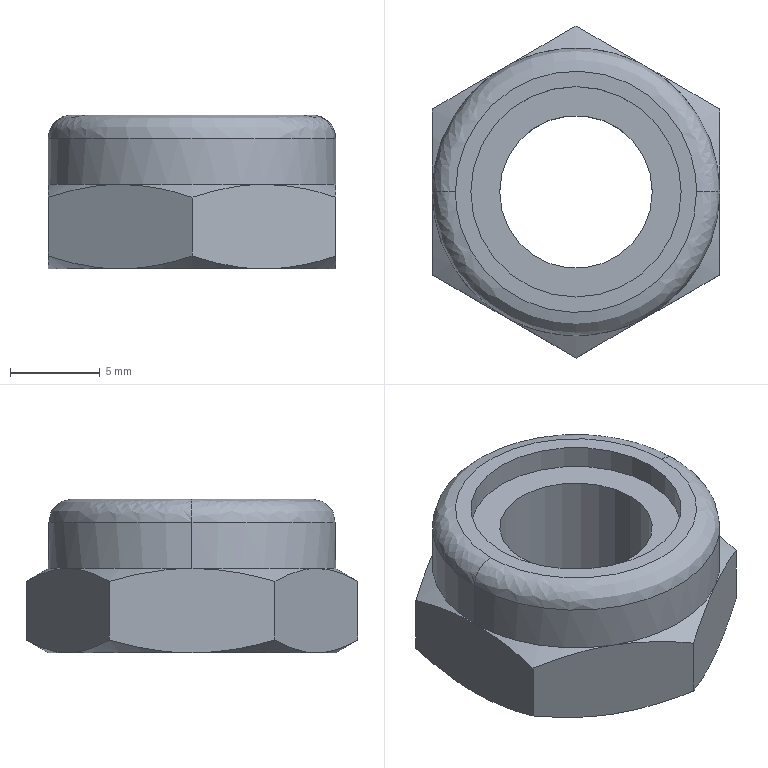Part | STEP file | Microwave Drying Flat Conveyor-prevailing torque nut thin insert_din_DIN EN ISO 10511 - M10 - N_Default | 1 solid | 33 faces | box 16 x 18.475 x 8.56 mm | volume 1235 mm3 | cone 14 | plane 9 | cylinder 8 | spline 2 | commonest cylinder face diameters 8.5 x2 10 x2 11.714 x2 16 x2
STEP:
#1=CARTESIAN_POINT('',(6.713,0.,3.86));
#2=VERTEX_POINT('',#1);
#3=CARTESIAN_POINT('',(-6.713,0.,3.86));
#4=VERTEX_POINT('',#3);
#5=CARTESIAN_POINT('',(6.713,0.,3.86));
#6=CARTESIAN_POINT('',(6.713,-13.427,3.86));
#7=CARTESIAN_POINT('',(-6.713,-13.427,3.86));
#8=CARTESIAN_POINT('',(-6.713,0.,3.86));
#9=(BOUNDED_CURVE()B_SPLINE_CURVE(3,(#5,#6,#7,#8),.UNSPECIFIED.,.F.,.F.)B_SPLINE_CURVE_WITH_KNOTS((4,4),(0.,1.),.UNSPECIFIED.)CURVE()GEOMETRIC_REPRESENTATION_ITEM()RATIONAL_B_SPLINE_CURVE((1.,0.3333,0.3333,1.))REPRESENTATION_ITEM(''));
#10=EDGE_CURVE('',#2,#4,#9,.T.);
#11=ORIENTED_EDGE('',*,*,#10,.T.);
#12=CARTESIAN_POINT('',(-8.,0.,2.573));
#13=VERTEX_POINT('',#12);
#14=CARTESIAN_POINT('',(-6.713,0.,2.573));
#15=DIRECTION('',(0.,-1.,0.));
#16=DIRECTION('',(-1.,0.,0.));
#17=AXIS2_PLACEMENT_3D('',#14,#15,#16);
#18=CIRCLE('',#17,1.287);
#19=EDGE_CURVE('',#4,#13,#18,.T.);
#20=ORIENTED_EDGE('',*,*,#19,.T.);
#21=CARTESIAN_POINT('',(8.,0.,2.573));
#22=VERTEX_POINT('',#21);
#23=CARTESIAN_POINT('',(0.,0.,2.573));
#24=DIRECTION('',(0.,0.,-1.));
#25=DIRECTION('',(1.,0.,0.));
#26=AXIS2_PLACEMENT_3D('',#23,#24,#25);
#27=CIRCLE('',#26,8.);
#28=EDGE_CURVE('',#22,#13,#27,.T.);
#29=ORIENTED_EDGE('',*,*,#28,.F.);
#30=CARTESIAN_POINT('',(6.713,0.,2.573));
#31=DIRECTION('',(0.,1.,0.));
#32=DIRECTION('',(1.,0.,0.));
#33=AXIS2_PLACEMENT_3D('',#30,#31,#32);
#34=CIRCLE('',#33,1.287);
#35=EDGE_CURVE('',#2,#22,#34,.T.);
#36=ORIENTED_EDGE('',*,*,#35,.F.);
#37=EDGE_LOOP('',(#11,#20,#29,#36));
#38=FACE_OUTER_BOUND('',#37,.T.);
#39=CARTESIAN_POINT('',(-6.713,0.,3.86));
#40=CARTESIAN_POINT('',(-6.713,-13.427,3.86));
#41=CARTESIAN_POINT('',(6.713,-13.427,3.86));
#42=CARTESIAN_POINT('',(6.713,0.,3.86));
#43=CARTESIAN_POINT('',(-7.467,0.,3.86));
#44=CARTESIAN_POINT('',(-7.467,-14.934,3.86));
#45=CARTESIAN_POINT('',(7.467,-14.934,3.86));
#46=CARTESIAN_POINT('',(7.467,0.,3.86));
#47=CARTESIAN_POINT('',(-8.,0.,3.327));
#48=CARTESIAN_POINT('',(-8.,-16.,3.327));
#49=CARTESIAN_POINT('',(8.,-16.,3.327));
#50=CARTESIAN_POINT('',(8.,0.,3.327));
#51=CARTESIAN_POINT('',(-8.,0.,2.573));
#52=CARTESIAN_POINT('',(-8.,-16.,2.573));
#53=CARTESIAN_POINT('',(8.,-16.,2.573));
#54=CARTESIAN_POINT('',(8.,0.,2.573));
#55=(BOUNDED_SURFACE()B_SPLINE_SURFACE(3,3,((#39,#40,#41,#42),(#43,#44,#45,#46),(#47,#48,#49,#50),(#51,#52,#53,#54)),.UNSPECIFIED.,.F.,.F.,.F.)B_SPLINE_SURFACE_WITH_KNOTS((4,4),(4,4),(0.,1.),(0.,1.),.UNSPECIFIED.)GEOMETRIC_REPRESENTATION_ITEM()RATIONAL_B_SPLINE_SURFACE(((1.,0.3333,0.3333,1.),(0.8047,0.2682,0.2682,0.8047),(0.8047,0.2682,0.2682,0.8047),(1.,0.3333,0.3333,1.)))REPRESENTATION_ITEM('')SURFACE());
#56=ADVANCED_FACE('',(#38),#55,.T.);
#57=CARTESIAN_POINT('',(-5.,0.,-4.7));
#58=VERTEX_POINT('',#57);
#59=CARTESIAN_POINT('',(5.,0.,-4.7));
#60=VERTEX_POINT('',#59);
#61=CARTESIAN_POINT('',(0.,0.,-4.7));
#62=DIRECTION('',(0.,0.,1.));
#63=DIRECTION('',(1.,0.,0.));
#64=AXIS2_PLACEMENT_3D('',#61,#62,#63);
#65=CIRCLE('',#64,5.);
#66=EDGE_CURVE('',#58,#60,#65,.T.);
#67=ORIENTED_EDGE('',*,*,#66,.F.);
#68=CARTESIAN_POINT('',(-5.,0.,-4.675));
#69=VERTEX_POINT('',#68);
#70=CARTESIAN_POINT('',(-5.,0.,19.05));
#71=DIRECTION('',(0.,0.,1.));
#72=VECTOR('',#71,1000.);
#73=LINE('',#70,#72);
#74=EDGE_CURVE('',#58,#69,#73,.T.);
#75=ORIENTED_EDGE('',*,*,#74,.T.);
#76=CARTESIAN_POINT('',(5.,0.,-4.675));
#77=VERTEX_POINT('',#76);
#78=CARTESIAN_POINT('',(0.,0.,-4.675));
#79=DIRECTION('',(0.,0.,-1.));
#80=DIRECTION('',(1.,0.,0.));
#81=AXIS2_PLACEMENT_3D('',#78,#79,#80);
#82=CIRCLE('',#81,5.);
#83=EDGE_CURVE('',#77,#69,#82,.T.);
#84=ORIENTED_EDGE('',*,*,#83,.F.);
#85=CARTESIAN_POINT('',(5.,0.,19.05));
#86=DIRECTION('',(0.,0.,1.));
#87=VECTOR('',#86,1000.);
#88=LINE('',#85,#87);
#89=EDGE_CURVE('',#60,#77,#88,.T.);
#90=ORIENTED_EDGE('',*,*,#89,.F.);
#91=EDGE_LOOP('',(#67,#75,#84,#90));
#92=FACE_OUTER_BOUND('',#91,.T.);
#93=CARTESIAN_POINT('',(0.,0.,19.05));
#94=DIRECTION('',(0.,0.,1.));
#95=DIRECTION('',(1.,0.,0.));
#96=AXIS2_PLACEMENT_3D('',#93,#94,#95);
#97=CYLINDRICAL_SURFACE('',#96,5.);
#98=ADVANCED_FACE('',(#92),#97,.F.);
#99=CARTESIAN_POINT('',(4.25,0.,-4.149));
#100=VERTEX_POINT('',#99);
#101=CARTESIAN_POINT('',(-4.25,0.,-4.149));
#102=VERTEX_POINT('',#101);
#103=CARTESIAN_POINT('',(0.,0.,-4.149));
#104=DIRECTION('',(0.,0.,-1.));
#105=DIRECTION('',(-1.,0.,0.));
#106=AXIS2_PLACEMENT_3D('',#103,#104,#105);
#107=CIRCLE('',#106,4.25);
#108=EDGE_CURVE('',#100,#102,#107,.T.);
#109=ORIENTED_EDGE('',*,*,#108,.F.);
#110=CARTESIAN_POINT('',(5.,0.,-4.675));
#111=DIRECTION('',(0.8192,0.,-0.5736));
#112=VECTOR('',#111,1000.);
#113=LINE('',#110,#112);
#114=EDGE_CURVE('',#100,#77,#113,.T.);
#115=ORIENTED_EDGE('',*,*,#114,.T.);
#116=ORIENTED_EDGE('',*,*,#83,.T.);
#117=CARTESIAN_POINT('',(-5.,0.,-4.675));
#118=DIRECTION('',(-0.8192,0.,-0.5736));
#119=VECTOR('',#118,1000.);
#120=LINE('',#117,#119);
#121=EDGE_CURVE('',#102,#69,#120,.T.);
#122=ORIENTED_EDGE('',*,*,#121,.F.);
#123=EDGE_LOOP('',(#109,#115,#116,#122));
#124=FACE_OUTER_BOUND('',#123,.T.);
#125=CARTESIAN_POINT('',(0.,0.,-4.675));
#126=DIRECTION('',(0.,0.,-1.));
#127=DIRECTION('',(-1.,0.,0.));
#128=AXIS2_PLACEMENT_3D('',#125,#126,#127);
#129=CONICAL_SURFACE('',#128,5.,0.9599);
#130=ADVANCED_FACE('',(#124),#129,.F.);
#131=ORIENTED_EDGE('',*,*,#108,.T.);
#132=CARTESIAN_POINT('',(-4.25,0.,2.573));
#133=VERTEX_POINT('',#132);
#134=CARTESIAN_POINT('',(-4.25,0.,-4.7));
#135=DIRECTION('',(0.,0.,1.));
#136=VECTOR('',#135,1000.);
#137=LINE('',#134,#136);
#138=EDGE_CURVE('',#102,#133,#137,.T.);
#139=ORIENTED_EDGE('',*,*,#138,.T.);
#140=CARTESIAN_POINT('',(4.25,0.,2.573));
#141=VERTEX_POINT('',#140);
#142=CARTESIAN_POINT('',(0.,0.,2.573));
#143=DIRECTION('',(0.,0.,-1.));
#144=DIRECTION('',(1.,0.,0.));
#145=AXIS2_PLACEMENT_3D('',#142,#143,#144);
#146=CIRCLE('',#145,4.25);
#147=EDGE_CURVE('',#141,#133,#146,.T.);
#148=ORIENTED_EDGE('',*,*,#147,.F.);
#149=CARTESIAN_POINT('',(4.25,0.,-4.7));
#150=DIRECTION('',(0.,0.,1.));
#151=VECTOR('',#150,1000.);
#152=LINE('',#149,#151);
#153=EDGE_CURVE('',#100,#141,#152,.T.);
#154=ORIENTED_EDGE('',*,*,#153,.F.);
#155=EDGE_LOOP('',(#131,#139,#148,#154));
#156=FACE_OUTER_BOUND('',#155,.T.);
#157=CARTESIAN_POINT('',(0.,0.,-4.7));
#158=DIRECTION('',(0.,0.,1.));
#159=DIRECTION('',(1.,0.,0.));
#160=AXIS2_PLACEMENT_3D('',#157,#158,#159);
#161=CYLINDRICAL_SURFACE('',#160,4.25);
#162=ADVANCED_FACE('',(#156),#161,.F.);
#163=CARTESIAN_POINT('',(-8.,0.,0.));
#164=VERTEX_POINT('',#163);
#165=CARTESIAN_POINT('',(-4.,6.928,0.));
#166=VERTEX_POINT('',#165);
#167=CARTESIAN_POINT('',(0.,0.,0.));
#168=DIRECTION('',(0.,0.,-1.));
#169=DIRECTION('',(-1.,0.,0.));
#170=AXIS2_PLACEMENT_3D('',#167,#168,#169);
#171=CIRCLE('',#170,8.);
#172=EDGE_CURVE('',#164,#166,#171,.T.);
#173=ORIENTED_EDGE('',*,*,#172,.F.);
#174=CARTESIAN_POINT('',(-8.,0.,9.481));
#175=DIRECTION('',(0.,0.,1.));
#176=VECTOR('',#175,1000.);
#177=LINE('',#174,#176);
#178=EDGE_CURVE('',#164,#13,#177,.T.);
#179=ORIENTED_EDGE('',*,*,#178,.T.);
#180=CARTESIAN_POINT('',(0.,0.,2.573));
#181=DIRECTION('',(0.,0.,-1.));
#182=DIRECTION('',(1.,0.,0.));
#183=AXIS2_PLACEMENT_3D('',#180,#181,#182);
#184=CIRCLE('',#183,8.);
#185=EDGE_CURVE('',#13,#22,#184,.T.);
#186=ORIENTED_EDGE('',*,*,#185,.T.);
#187=CARTESIAN_POINT('',(8.,0.,0.));
#188=VERTEX_POINT('',#187);
#189=CARTESIAN_POINT('',(8.,0.,9.481));
#190=DIRECTION('',(0.,0.,1.));
#191=VECTOR('',#190,1000.);
#192=LINE('',#189,#191);
#193=EDGE_CURVE('',#188,#22,#192,.T.);
#194=ORIENTED_EDGE('',*,*,#193,.F.);
#195=CARTESIAN_POINT('',(4.,6.928,0.));
#196=VERTEX_POINT('',#195);
#197=CARTESIAN_POINT('',(0.,0.,0.));
#198=DIRECTION('',(0.,0.,-1.));
#199=DIRECTION('',(-1.,0.,0.));
#200=AXIS2_PLACEMENT_3D('',#197,#198,#199);
#201=CIRCLE('',#200,8.);
#202=EDGE_CURVE('',#196,#188,#201,.T.);
#203=ORIENTED_EDGE('',*,*,#202,.F.);
#204=CARTESIAN_POINT('',(0.,0.,0.));
#205=DIRECTION('',(0.,0.,-1.));
#206=DIRECTION('',(-1.,0.,0.));
#207=AXIS2_PLACEMENT_3D('',#204,#205,#206);
#208=CIRCLE('',#207,8.);
#209=EDGE_CURVE('',#166,#196,#208,.T.);
#210=ORIENTED_EDGE('',*,*,#209,.F.);
#211=EDGE_LOOP('',(#173,#179,#186,#194,#203,#210));
#212=FACE_OUTER_BOUND('',#211,.T.);
#213=CARTESIAN_POINT('',(0.,0.,9.481));
#214=DIRECTION('',(0.,0.,1.));
#215=DIRECTION('',(1.,0.,0.));
#216=AXIS2_PLACEMENT_3D('',#213,#214,#215);
#217=CYLINDRICAL_SURFACE('',#216,8.);
#218=ADVANCED_FACE('',(#212),#217,.T.);
#219=CARTESIAN_POINT('',(5.857,0.,2.573));
#220=VERTEX_POINT('',#219);
#221=CARTESIAN_POINT('',(-5.857,0.,2.573));
#222=VERTEX_POINT('',#221);
#223=CARTESIAN_POINT('',(0.,0.,2.573));
#224=DIRECTION('',(0.,0.,-1.));
#225=DIRECTION('',(1.,0.,0.));
#226=AXIS2_PLACEMENT_3D('',#223,#224,#225);
#227=CIRCLE('',#226,5.857);
#228=EDGE_CURVE('',#220,#222,#227,.T.);
#229=ORIENTED_EDGE('',*,*,#228,.T.);
#230=CARTESIAN_POINT('',(-5.857,0.,3.86));
#231=VERTEX_POINT('',#230);
#232=CARTESIAN_POINT('',(-5.857,0.,9.481));
#233=DIRECTION('',(0.,0.,1.));
#234=VECTOR('',#233,1000.);
#235=LINE('',#232,#234);
#236=EDGE_CURVE('',#222,#231,#235,.T.);
#237=ORIENTED_EDGE('',*,*,#236,.T.);
#238=CARTESIAN_POINT('',(5.857,0.,3.86));
#239=VERTEX_POINT('',#238);
#240=CARTESIAN_POINT('',(0.,0.,3.86));
#241=DIRECTION('',(0.,0.,-1.));
#242=DIRECTION('',(1.,0.,0.));
#243=AXIS2_PLACEMENT_3D('',#240,#241,#242);
#244=CIRCLE('',#243,5.857);
#245=EDGE_CURVE('',#239,#231,#244,.T.);
#246=ORIENTED_EDGE('',*,*,#245,.F.);
#247=CARTESIAN_POINT('',(5.857,0.,9.481));
#248=DIRECTION('',(0.,0.,1.));
#249=VECTOR('',#248,1000.);
#250=LINE('',#247,#249);
#251=EDGE_CURVE('',#220,#239,#250,.T.);
#252=ORIENTED_EDGE('',*,*,#251,.F.);
#253=EDGE_LOOP('',(#229,#237,#246,#252));
#254=FACE_OUTER_BOUND('',#253,.T.);
#255=CARTESIAN_POINT('',(0.,0.,9.481));
#256=DIRECTION('',(0.,0.,1.));
#257=DIRECTION('',(1.,0.,0.));
#258=AXIS2_PLACEMENT_3D('',#255,#256,#257);
#259=CYLINDRICAL_SURFACE('',#258,5.857);
#260=ADVANCED_FACE('',(#254),#259,.F.);
#261=CARTESIAN_POINT('',(8.,0.,-4.7));
#262=VERTEX_POINT('',#261);
#263=CARTESIAN_POINT('',(4.,-6.928,-4.7));
#264=VERTEX_POINT('',#263);
#265=CARTESIAN_POINT('',(0.,0.,-4.7));
#266=DIRECTION('',(0.,0.,-1.));
#267=DIRECTION('',(1.,0.,0.));
#268=AXIS2_PLACEMENT_3D('',#265,#266,#267);
#269=CIRCLE('',#268,8.);
#270=EDGE_CURVE('',#262,#264,#269,.T.);
#271=ORIENTED_EDGE('',*,*,#270,.T.);
#272=CARTESIAN_POINT('',(-4.,-6.928,-4.7));
#273=VERTEX_POINT('',#272);
#274=CARTESIAN_POINT('',(0.,0.,-4.7));
#275=DIRECTION('',(0.,0.,-1.));
#276=DIRECTION('',(1.,0.,0.));
#277=AXIS2_PLACEMENT_3D('',#274,#275,#276);
#278=CIRCLE('',#277,8.);
#279=EDGE_CURVE('',#264,#273,#278,.T.);
#280=ORIENTED_EDGE('',*,*,#279,.T.);
#281=CARTESIAN_POINT('',(-8.,0.,-4.7));
#282=VERTEX_POINT('',#281);
#283=CARTESIAN_POINT('',(0.,0.,-4.7));
#284=DIRECTION('',(0.,0.,-1.));
#285=DIRECTION('',(1.,0.,0.));
#286=AXIS2_PLACEMENT_3D('',#283,#284,#285);
#287=CIRCLE('',#286,8.);
#288=EDGE_CURVE('',#273,#282,#287,.T.);
#289=ORIENTED_EDGE('',*,*,#288,.T.);
#290=CARTESIAN_POINT('',(-4.,6.928,-4.7));
#291=VERTEX_POINT('',#290);
#292=CARTESIAN_POINT('',(0.,0.,-4.7));
#293=DIRECTION('',(0.,0.,-1.));
#294=DIRECTION('',(1.,0.,0.));
#295=AXIS2_PLACEMENT_3D('',#292,#293,#294);
#296=CIRCLE('',#295,8.);
#297=EDGE_CURVE('',#282,#291,#296,.T.);
#298=ORIENTED_EDGE('',*,*,#297,.T.);
#299=CARTESIAN_POINT('',(4.,6.928,-4.7));
#300=VERTEX_POINT('',#299);
#301=CARTESIAN_POINT('',(0.,0.,-4.7));
#302=DIRECTION('',(0.,0.,-1.));
#303=DIRECTION('',(1.,0.,0.));
#304=AXIS2_PLACEMENT_3D('',#301,#302,#303);
#305=CIRCLE('',#304,8.);
#306=EDGE_CURVE('',#291,#300,#305,.T.);
#307=ORIENTED_EDGE('',*,*,#306,.T.);
#308=CARTESIAN_POINT('',(0.,0.,-4.7));
#309=DIRECTION('',(0.,0.,-1.));
#310=DIRECTION('',(1.,0.,0.));
#311=AXIS2_PLACEMENT_3D('',#308,#309,#310);
#312=CIRCLE('',#311,8.);
#313=EDGE_CURVE('',#300,#262,#312,.T.);
#314=ORIENTED_EDGE('',*,*,#313,.T.);
#315=EDGE_LOOP('',(#271,#280,#289,#298,#307,#314));
#316=FACE_OUTER_BOUND('',#315,.T.);
#317=CARTESIAN_POINT('',(0.,0.,-4.7));
#318=DIRECTION('',(0.,0.,1.));
#319=DIRECTION('',(1.,0.,0.));
#320=AXIS2_PLACEMENT_3D('',#317,#318,#319);
#321=CIRCLE('',#320,5.);
#322=EDGE_CURVE('',#60,#58,#321,.T.);
#323=ORIENTED_EDGE('',*,*,#322,.T.);
#324=ORIENTED_EDGE('',*,*,#66,.T.);
#325=EDGE_LOOP('',(#323,#324));
#326=FACE_BOUND('',#325,.T.);
#327=CARTESIAN_POINT('',(0.,9.238,-4.7));
#328=DIRECTION('',(0.,0.,-1.));
#329=DIRECTION('',(-1.,0.,0.));
#330=AXIS2_PLACEMENT_3D('',#327,#328,#329);
#331=PLANE('',#330);
#332=ADVANCED_FACE('',(#316,#326),#331,.T.);
#333=CARTESIAN_POINT('',(0.000000014,-9.238,-3.985));
#334=VERTEX_POINT('',#333);
#335=CARTESIAN_POINT('',(0.000000014,-9.238,-3.985));
#336=CARTESIAN_POINT('',(-0.6534,-8.86,-4.203));
#337=CARTESIAN_POINT('',(-1.312,-8.48,-4.383));
#338=CARTESIAN_POINT('',(-2.644,-7.711,-4.632));
#339=CARTESIAN_POINT('',(-3.317,-7.322,-4.7));
#340=CARTESIAN_POINT('',(-4.,-6.928,-4.7));
#341=B_SPLINE_CURVE_WITH_KNOTS('',3,(#335,#336,#337,#338,#339,#340),.UNSPECIFIED.,.F.,.F.,(4,2,4),(0.,0.002337,0.004674),.UNSPECIFIED.);
#342=EDGE_CURVE('',#334,#273,#341,.T.);
#343=ORIENTED_EDGE('',*,*,#342,.T.);
#344=ORIENTED_EDGE('',*,*,#279,.F.);
#345=CARTESIAN_POINT('',(4.,-6.928,-4.7));
#346=CARTESIAN_POINT('',(3.317,-7.322,-4.7));
#347=CARTESIAN_POINT('',(2.644,-7.711,-4.632));
#348=CARTESIAN_POINT('',(1.312,-8.48,-4.383));
#349=CARTESIAN_POINT('',(0.6534,-8.86,-4.203));
#350=CARTESIAN_POINT('',(0.000000014,-9.238,-3.985));
#351=B_SPLINE_CURVE_WITH_KNOTS('',3,(#345,#346,#347,#348,#349,#350),.UNSPECIFIED.,.F.,.F.,(4,2,4),(0.,0.002337,0.004674),.UNSPECIFIED.);
#352=EDGE_CURVE('',#264,#334,#351,.T.);
#353=ORIENTED_EDGE('',*,*,#352,.T.);
#354=EDGE_LOOP('',(#343,#344,#353));
#355=FACE_OUTER_BOUND('',#354,.T.);
#356=CARTESIAN_POINT('',(0.,0.,-3.981));
#357=DIRECTION('',(0.,0.,1.));
#358=DIRECTION('',(1.,0.,0.));
#359=AXIS2_PLACEMENT_3D('',#356,#357,#358);
#360=CONICAL_SURFACE('',#359,9.245,1.047);
#361=ADVANCED_FACE('',(#355),#360,.T.);
#362=ORIENTED_EDGE('',*,*,#270,.F.);
#363=CARTESIAN_POINT('',(8.,-4.619,-3.985));
#364=VERTEX_POINT('',#363);
#365=CARTESIAN_POINT('',(8.,0.,-4.7));
#366=CARTESIAN_POINT('',(8.,-0.7882,-4.7));
#367=CARTESIAN_POINT('',(8.,-1.566,-4.632));
#368=CARTESIAN_POINT('',(8.,-3.104,-4.383));
#369=CARTESIAN_POINT('',(8.,-3.864,-4.203));
#370=CARTESIAN_POINT('',(8.,-4.619,-3.985));
#371=B_SPLINE_CURVE_WITH_KNOTS('',3,(#365,#366,#367,#368,#369,#370),.UNSPECIFIED.,.F.,.F.,(4,2,4),(0.,0.002337,0.004674),.UNSPECIFIED.);
#372=EDGE_CURVE('',#262,#364,#371,.T.);
#373=ORIENTED_EDGE('',*,*,#372,.T.);
#374=CARTESIAN_POINT('',(8.,-4.619,-3.985));
#375=CARTESIAN_POINT('',(7.347,-4.996,-4.203));
#376=CARTESIAN_POINT('',(6.688,-5.376,-4.383));
#377=CARTESIAN_POINT('',(5.356,-6.145,-4.632));
#378=CARTESIAN_POINT('',(4.683,-6.534,-4.7));
#379=CARTESIAN_POINT('',(4.,-6.928,-4.7));
#380=B_SPLINE_CURVE_WITH_KNOTS('',3,(#374,#375,#376,#377,#378,#379),.UNSPECIFIED.,.F.,.F.,(4,2,4),(0.,0.002337,0.004674),.UNSPECIFIED.);
#381=EDGE_CURVE('',#364,#264,#380,.T.);
#382=ORIENTED_EDGE('',*,*,#381,.T.);
#383=EDGE_LOOP('',(#362,#373,#382));
#384=FACE_OUTER_BOUND('',#383,.T.);
#385=CARTESIAN_POINT('',(0.,0.,-3.981));
#386=DIRECTION('',(0.,0.,1.));
#387=DIRECTION('',(1.,0.,0.));
#388=AXIS2_PLACEMENT_3D('',#385,#386,#387);
#389=CONICAL_SURFACE('',#388,9.245,1.047);
#390=ADVANCED_FACE('',(#384),#389,.T.);
#391=CARTESIAN_POINT('',(8.,4.619,-3.985));
#392=VERTEX_POINT('',#391);
#393=CARTESIAN_POINT('',(8.,4.619,-3.985));
#394=CARTESIAN_POINT('',(8.,3.864,-4.203));
#395=CARTESIAN_POINT('',(8.,3.104,-4.383));
#396=CARTESIAN_POINT('',(8.,1.566,-4.632));
#397=CARTESIAN_POINT('',(8.,0.7882,-4.7));
#398=CARTESIAN_POINT('',(8.,0.,-4.7));
#399=B_SPLINE_CURVE_WITH_KNOTS('',3,(#393,#394,#395,#396,#397,#398),.UNSPECIFIED.,.F.,.F.,(4,2,4),(0.,0.002337,0.004674),.UNSPECIFIED.);
#400=EDGE_CURVE('',#392,#262,#399,.T.);
#401=ORIENTED_EDGE('',*,*,#400,.T.);
#402=ORIENTED_EDGE('',*,*,#313,.F.);
#403=CARTESIAN_POINT('',(4.,6.928,-4.7));
#404=CARTESIAN_POINT('',(4.683,6.534,-4.7));
#405=CARTESIAN_POINT('',(5.356,6.145,-4.632));
#406=CARTESIAN_POINT('',(6.688,5.376,-4.383));
#407=CARTESIAN_POINT('',(7.347,4.996,-4.203));
#408=CARTESIAN_POINT('',(8.,4.619,-3.985));
#409=B_SPLINE_CURVE_WITH_KNOTS('',3,(#403,#404,#405,#406,#407,#408),.UNSPECIFIED.,.F.,.F.,(4,2,4),(0.,0.002337,0.004674),.UNSPECIFIED.);
#410=EDGE_CURVE('',#300,#392,#409,.T.);
#411=ORIENTED_EDGE('',*,*,#410,.T.);
#412=EDGE_LOOP('',(#401,#402,#411));
#413=FACE_OUTER_BOUND('',#412,.T.);
#414=CARTESIAN_POINT('',(0.,0.,-3.981));
#415=DIRECTION('',(0.,0.,1.));
#416=DIRECTION('',(1.,0.,0.));
#417=AXIS2_PLACEMENT_3D('',#414,#415,#416);
#418=CONICAL_SURFACE('',#417,9.245,1.047);
#419=ADVANCED_FACE('',(#413),#418,.T.);
#420=CARTESIAN_POINT('',(-0.000000014,9.238,-3.985));
#421=VERTEX_POINT('',#420);
#422=CARTESIAN_POINT('',(-0.000000014,9.238,-3.985));
#423=CARTESIAN_POINT('',(0.6534,8.86,-4.203));
#424=CARTESIAN_POINT('',(1.312,8.48,-4.383));
#425=CARTESIAN_POINT('',(2.644,7.711,-4.632));
#426=CARTESIAN_POINT('',(3.317,7.322,-4.7));
#427=CARTESIAN_POINT('',(4.,6.928,-4.7));
#428=B_SPLINE_CURVE_WITH_KNOTS('',3,(#422,#423,#424,#425,#426,#427),.UNSPECIFIED.,.F.,.F.,(4,2,4),(0.,0.002337,0.004674),.UNSPECIFIED.);
#429=EDGE_CURVE('',#421,#300,#428,.T.);
#430=ORIENTED_EDGE('',*,*,#429,.T.);
#431=ORIENTED_EDGE('',*,*,#306,.F.);
#432=CARTESIAN_POINT('',(-4.,6.928,-4.7));
#433=CARTESIAN_POINT('',(-3.317,7.322,-4.7));
#434=CARTESIAN_POINT('',(-2.644,7.711,-4.632));
#435=CARTESIAN_POINT('',(-1.312,8.48,-4.383));
#436=CARTESIAN_POINT('',(-0.6534,8.86,-4.203));
#437=CARTESIAN_POINT('',(-0.000000014,9.238,-3.985));
#438=B_SPLINE_CURVE_WITH_KNOTS('',3,(#432,#433,#434,#435,#436,#437),.UNSPECIFIED.,.F.,.F.,(4,2,4),(0.,0.002337,0.004674),.UNSPECIFIED.);
#439=EDGE_CURVE('',#291,#421,#438,.T.);
#440=ORIENTED_EDGE('',*,*,#439,.T.);
#441=EDGE_LOOP('',(#430,#431,#440));
#442=FACE_OUTER_BOUND('',#441,.T.);
#443=CARTESIAN_POINT('',(0.,0.,-3.981));
#444=DIRECTION('',(0.,0.,1.));
#445=DIRECTION('',(1.,0.,0.));
#446=AXIS2_PLACEMENT_3D('',#443,#444,#445);
#447=CONICAL_SURFACE('',#446,9.245,1.047);
#448=ADVANCED_FACE('',(#442),#447,.T.);
#449=ORIENTED_EDGE('',*,*,#297,.F.);
#450=CARTESIAN_POINT('',(-8.,4.619,-3.985));
#451=VERTEX_POINT('',#450);
#452=CARTESIAN_POINT('',(-8.,0.,-4.7));
#453=CARTESIAN_POINT('',(-8.,0.7882,-4.7));
#454=CARTESIAN_POINT('',(-8.,1.566,-4.632));
#455=CARTESIAN_POINT('',(-8.,3.104,-4.383));
#456=CARTESIAN_POINT('',(-8.,3.864,-4.203));
#457=CARTESIAN_POINT('',(-8.,4.619,-3.985));
#458=B_SPLINE_CURVE_WITH_KNOTS('',3,(#452,#453,#454,#455,#456,#457),.UNSPECIFIED.,.F.,.F.,(4,2,4),(0.,0.002337,0.004674),.UNSPECIFIED.);
#459=EDGE_CURVE('',#282,#451,#458,.T.);
#460=ORIENTED_EDGE('',*,*,#459,.T.);
#461=CARTESIAN_POINT('',(-8.,4.619,-3.985));
#462=CARTESIAN_POINT('',(-7.347,4.996,-4.203));
#463=CARTESIAN_POINT('',(-6.688,5.376,-4.383));
#464=CARTESIAN_POINT('',(-5.356,6.145,-4.632));
#465=CARTESIAN_POINT('',(-4.683,6.534,-4.7));
#466=CARTESIAN_POINT('',(-4.,6.928,-4.7));
#467=B_SPLINE_CURVE_WITH_KNOTS('',3,(#461,#462,#463,#464,#465,#466),.UNSPECIFIED.,.F.,.F.,(4,2,4),(0.,0.002337,0.004674),.UNSPECIFIED.);
#468=EDGE_CURVE('',#451,#291,#467,.T.);
#469=ORIENTED_EDGE('',*,*,#468,.T.);
#470=EDGE_LOOP('',(#449,#460,#469));
#471=FACE_OUTER_BOUND('',#470,.T.);
#472=CARTESIAN_POINT('',(0.,0.,-3.981));
#473=DIRECTION('',(0.,0.,1.));
#474=DIRECTION('',(1.,0.,0.));
#475=AXIS2_PLACEMENT_3D('',#472,#473,#474);
#476=CONICAL_SURFACE('',#475,9.245,1.047);
#477=ADVANCED_FACE('',(#471),#476,.T.);
#478=CARTESIAN_POINT('',(-8.,-4.619,-3.985));
#479=VERTEX_POINT('',#478);
#480=CARTESIAN_POINT('',(-8.,-4.619,-3.985));
#481=CARTESIAN_POINT('',(-8.,-3.864,-4.203));
#482=CARTESIAN_POINT('',(-8.,-3.104,-4.383));
#483=CARTESIAN_POINT('',(-8.,-1.566,-4.632));
#484=CARTESIAN_POINT('',(-8.,-0.7882,-4.7));
#485=CARTESIAN_POINT('',(-8.,0.,-4.7));
#486=B_SPLINE_CURVE_WITH_KNOTS('',3,(#480,#481,#482,#483,#484,#485),.UNSPECIFIED.,.F.,.F.,(4,2,4),(0.,0.002337,0.004674),.UNSPECIFIED.);
#487=EDGE_CURVE('',#479,#282,#486,.T.);
#488=ORIENTED_EDGE('',*,*,#487,.T.);
#489=ORIENTED_EDGE('',*,*,#288,.F.);
#490=CARTESIAN_POINT('',(-4.,-6.928,-4.7));
#491=CARTESIAN_POINT('',(-4.683,-6.534,-4.7));
#492=CARTESIAN_POINT('',(-5.356,-6.145,-4.632));
#493=CARTESIAN_POINT('',(-6.688,-5.376,-4.383));
#494=CARTESIAN_POINT('',(-7.347,-4.996,-4.203));
#495=CARTESIAN_POINT('',(-8.,-4.619,-3.985));
#496=B_SPLINE_CURVE_WITH_KNOTS('',3,(#490,#491,#492,#493,#494,#495),.UNSPECIFIED.,.F.,.F.,(4,2,4),(0.,0.002337,0.004674),.UNSPECIFIED.);
#497=EDGE_CURVE('',#273,#479,#496,.T.);
#498=ORIENTED_EDGE('',*,*,#497,.T.);
#499=EDGE_LOOP('',(#488,#489,#498));
#500=FACE_OUTER_BOUND('',#499,.T.);
#501=CARTESIAN_POINT('',(0.,0.,-3.981));
#502=DIRECTION('',(0.,0.,1.));
#503=DIRECTION('',(1.,0.,0.));
#504=AXIS2_PLACEMENT_3D('',#501,#502,#503);
#505=CONICAL_SURFACE('',#504,9.245,1.047);
#506=ADVANCED_FACE('',(#500),#505,.T.);
#507=ORIENTED_EDGE('',*,*,#74,.F.);
#508=ORIENTED_EDGE('',*,*,#322,.F.);
#509=ORIENTED_EDGE('',*,*,#89,.T.);
#510=CARTESIAN_POINT('',(0.,0.,-4.675));
#511=DIRECTION('',(0.,0.,-1.));
#512=DIRECTION('',(1.,0.,0.));
#513=AXIS2_PLACEMENT_3D('',#510,#511,#512);
#514=CIRCLE('',#513,5.);
#515=EDGE_CURVE('',#69,#77,#514,.T.);
#516=ORIENTED_EDGE('',*,*,#515,.F.);
#517=EDGE_LOOP('',(#507,#508,#509,#516));
#518=FACE_OUTER_BOUND('',#517,.T.);
#519=CARTESIAN_POINT('',(0.,0.,19.05));
#520=DIRECTION('',(0.,0.,1.));
#521=DIRECTION('',(1.,0.,0.));
#522=AXIS2_PLACEMENT_3D('',#519,#520,#521);
#523=CYLINDRICAL_SURFACE('',#522,5.);
#524=ADVANCED_FACE('',(#518),#523,.F.);
#525=ORIENTED_EDGE('',*,*,#497,.F.);
#526=ORIENTED_EDGE('',*,*,#342,.F.);
#527=CARTESIAN_POINT('',(0.,-9.238,-0.7145));
#528=VERTEX_POINT('',#527);
#529=CARTESIAN_POINT('',(0.,-9.238,-4.7));
#530=DIRECTION('',(0.,0.,1.));
#531=VECTOR('',#530,1000.);
#532=LINE('',#529,#531);
#533=EDGE_CURVE('',#334,#528,#532,.T.);
#534=ORIENTED_EDGE('',*,*,#533,.T.);
#535=CARTESIAN_POINT('',(-4.,-6.928,0.));
#536=VERTEX_POINT('',#535);
#537=CARTESIAN_POINT('',(0.,-9.238,-0.7145));
#538=CARTESIAN_POINT('',(-0.6534,-8.86,-0.4967));
#539=CARTESIAN_POINT('',(-1.312,-8.48,-0.3171));
#540=CARTESIAN_POINT('',(-2.644,-7.711,-0.06831));
#541=CARTESIAN_POINT('',(-3.317,-7.322,0.));
#542=CARTESIAN_POINT('',(-4.,-6.928,0.));
#543=B_SPLINE_CURVE_WITH_KNOTS('',3,(#537,#538,#539,#540,#541,#542),.UNSPECIFIED.,.F.,.F.,(4,2,4),(0.,0.002337,0.004674),.UNSPECIFIED.);
#544=EDGE_CURVE('',#528,#536,#543,.T.);
#545=ORIENTED_EDGE('',*,*,#544,.T.);
#546=CARTESIAN_POINT('',(-8.,-4.619,-0.7145));
#547=VERTEX_POINT('',#546);
#548=CARTESIAN_POINT('',(-4.,-6.928,0.));
#549=CARTESIAN_POINT('',(-4.683,-6.534,0.));
#550=CARTESIAN_POINT('',(-5.356,-6.145,-0.06831));
#551=CARTESIAN_POINT('',(-6.688,-5.376,-0.3171));
#552=CARTESIAN_POINT('',(-7.347,-4.996,-0.4967));
#553=CARTESIAN_POINT('',(-8.,-4.619,-0.7145));
#554=B_SPLINE_CURVE_WITH_KNOTS('',3,(#548,#549,#550,#551,#552,#553),.UNSPECIFIED.,.F.,.F.,(4,2,4),(0.,0.002337,0.004674),.UNSPECIFIED.);
#555=EDGE_CURVE('',#536,#547,#554,.T.);
#556=ORIENTED_EDGE('',*,*,#555,.T.);
#557=CARTESIAN_POINT('',(-8.,-4.619,-4.7));
#558=DIRECTION('',(0.,0.,-1.));
#559=VECTOR('',#558,1000.);
#560=LINE('',#557,#559);
#561=EDGE_CURVE('',#547,#479,#560,.T.);
#562=ORIENTED_EDGE('',*,*,#561,.T.);
#563=EDGE_LOOP('',(#525,#526,#534,#545,#556,#562));
#564=FACE_OUTER_BOUND('',#563,.T.);
#565=CARTESIAN_POINT('',(-8.,-4.619,-4.7));
#566=DIRECTION('',(-0.5,-0.866,0.));
#567=DIRECTION('',(0.866,-0.5,0.));
#568=AXIS2_PLACEMENT_3D('',#565,#566,#567);
#569=PLANE('',#568);
#570=ADVANCED_FACE('',(#564),#569,.T.);
#571=ORIENTED_EDGE('',*,*,#352,.F.);
#572=ORIENTED_EDGE('',*,*,#381,.F.);
#573=CARTESIAN_POINT('',(8.,-4.619,-0.7145));
#574=VERTEX_POINT('',#573);
#575=CARTESIAN_POINT('',(8.,-4.619,-4.7));
#576=DIRECTION('',(0.,0.,1.));
#577=VECTOR('',#576,1000.);
#578=LINE('',#575,#577);
#579=EDGE_CURVE('',#364,#574,#578,.T.);
#580=ORIENTED_EDGE('',*,*,#579,.T.);
#581=CARTESIAN_POINT('',(4.,-6.928,0.));
#582=VERTEX_POINT('',#581);
#583=CARTESIAN_POINT('',(8.,-4.619,-0.7145));
#584=CARTESIAN_POINT('',(7.347,-4.996,-0.4967));
#585=CARTESIAN_POINT('',(6.688,-5.376,-0.3171));
#586=CARTESIAN_POINT('',(5.356,-6.145,-0.06831));
#587=CARTESIAN_POINT('',(4.683,-6.534,0.));
#588=CARTESIAN_POINT('',(4.,-6.928,0.));
#589=B_SPLINE_CURVE_WITH_KNOTS('',3,(#583,#584,#585,#586,#587,#588),.UNSPECIFIED.,.F.,.F.,(4,2,4),(0.,0.002337,0.004674),.UNSPECIFIED.);
#590=EDGE_CURVE('',#574,#582,#589,.T.);
#591=ORIENTED_EDGE('',*,*,#590,.T.);
#592=CARTESIAN_POINT('',(4.,-6.928,0.));
#593=CARTESIAN_POINT('',(3.317,-7.322,0.));
#594=CARTESIAN_POINT('',(2.644,-7.711,-0.06831));
#595=CARTESIAN_POINT('',(1.312,-8.48,-0.3171));
#596=CARTESIAN_POINT('',(0.6534,-8.86,-0.4967));
#597=CARTESIAN_POINT('',(0.,-9.238,-0.7145));
#598=B_SPLINE_CURVE_WITH_KNOTS('',3,(#592,#593,#594,#595,#596,#597),.UNSPECIFIED.,.F.,.F.,(4,2,4),(0.,0.002337,0.004674),.UNSPECIFIED.);
#599=EDGE_CURVE('',#582,#528,#598,.T.);
#600=ORIENTED_EDGE('',*,*,#599,.T.);
#601=ORIENTED_EDGE('',*,*,#533,.F.);
#602=EDGE_LOOP('',(#571,#572,#580,#591,#600,#601));
#603=FACE_OUTER_BOUND('',#602,.T.);
#604=CARTESIAN_POINT('',(0.,-9.238,-4.7));
#605=DIRECTION('',(0.5,-0.866,0.));
#606=DIRECTION('',(0.866,0.5,0.));
#607=AXIS2_PLACEMENT_3D('',#604,#605,#606);
#608=PLANE('',#607);
#609=ADVANCED_FACE('',(#603),#608,.T.);
#610=ORIENTED_EDGE('',*,*,#579,.F.);
#611=ORIENTED_EDGE('',*,*,#372,.F.);
#612=ORIENTED_EDGE('',*,*,#400,.F.);
#613=CARTESIAN_POINT('',(8.,4.619,-0.7145));
#614=VERTEX_POINT('',#613);
#615=CARTESIAN_POINT('',(8.,4.619,-4.7));
#616=DIRECTION('',(0.,0.,-1.));
#617=VECTOR('',#616,1000.);
#618=LINE('',#615,#617);
#619=EDGE_CURVE('',#614,#392,#618,.T.);
#620=ORIENTED_EDGE('',*,*,#619,.F.);
#621=CARTESIAN_POINT('',(8.,0.,0.));
#622=CARTESIAN_POINT('',(8.,0.7882,0.));
#623=CARTESIAN_POINT('',(8.,1.566,-0.06831));
#624=CARTESIAN_POINT('',(8.,3.104,-0.3171));
#625=CARTESIAN_POINT('',(8.,3.864,-0.4967));
#626=CARTESIAN_POINT('',(8.,4.619,-0.7145));
#627=B_SPLINE_CURVE_WITH_KNOTS('',3,(#621,#622,#623,#624,#625,#626),.UNSPECIFIED.,.F.,.F.,(4,2,4),(0.,0.002337,0.004674),.UNSPECIFIED.);
#628=EDGE_CURVE('',#188,#614,#627,.T.);
#629=ORIENTED_EDGE('',*,*,#628,.F.);
#630=CARTESIAN_POINT('',(8.,-4.619,-0.7145));
#631=CARTESIAN_POINT('',(8.,-3.864,-0.4967));
#632=CARTESIAN_POINT('',(8.,-3.104,-0.3171));
#633=CARTESIAN_POINT('',(8.,-1.566,-0.06831));
#634=CARTESIAN_POINT('',(8.,-0.7882,0.));
#635=CARTESIAN_POINT('',(8.,0.,0.));
#636=B_SPLINE_CURVE_WITH_KNOTS('',3,(#630,#631,#632,#633,#634,#635),.UNSPECIFIED.,.F.,.F.,(4,2,4),(0.,0.002337,0.004674),.UNSPECIFIED.);
#637=EDGE_CURVE('',#574,#188,#636,.T.);
#638=ORIENTED_EDGE('',*,*,#637,.F.);
#639=EDGE_LOOP('',(#610,#611,#612,#620,#629,#638));
#640=FACE_OUTER_BOUND('',#639,.T.);
#641=CARTESIAN_POINT('',(8.,4.619,-4.7));
#642=DIRECTION('',(-1.,0.,0.));
#643=DIRECTION('',(0.,0.,1.));
#644=AXIS2_PLACEMENT_3D('',#641,#642,#643);
#645=PLANE('',#644);
#646=ADVANCED_FACE('',(#640),#645,.F.);
#647=ORIENTED_EDGE('',*,*,#410,.F.);
#648=ORIENTED_EDGE('',*,*,#429,.F.);
#649=CARTESIAN_POINT('',(0.,9.238,-0.7145));
#650=VERTEX_POINT('',#649);
#651=CARTESIAN_POINT('',(0.,9.238,-4.7));
#652=DIRECTION('',(0.,0.,1.));
#653=VECTOR('',#652,1000.);
#654=LINE('',#651,#653);
#655=EDGE_CURVE('',#421,#650,#654,.T.);
#656=ORIENTED_EDGE('',*,*,#655,.T.);
#657=CARTESIAN_POINT('',(0.,9.238,-0.7145));
#658=CARTESIAN_POINT('',(0.6534,8.86,-0.4967));
#659=CARTESIAN_POINT('',(1.312,8.48,-0.3171));
#660=CARTESIAN_POINT('',(2.644,7.711,-0.06831));
#661=CARTESIAN_POINT('',(3.317,7.322,0.));
#662=CARTESIAN_POINT('',(4.,6.928,0.));
#663=B_SPLINE_CURVE_WITH_KNOTS('',3,(#657,#658,#659,#660,#661,#662),.UNSPECIFIED.,.F.,.F.,(4,2,4),(0.,0.002337,0.004674),.UNSPECIFIED.);
#664=EDGE_CURVE('',#650,#196,#663,.T.);
#665=ORIENTED_EDGE('',*,*,#664,.T.);
#666=CARTESIAN_POINT('',(4.,6.928,0.));
#667=CARTESIAN_POINT('',(4.683,6.534,0.));
#668=CARTESIAN_POINT('',(5.356,6.145,-0.06831));
#669=CARTESIAN_POINT('',(6.688,5.376,-0.3171));
#670=CARTESIAN_POINT('',(7.347,4.996,-0.4967));
#671=CARTESIAN_POINT('',(8.,4.619,-0.7145));
#672=B_SPLINE_CURVE_WITH_KNOTS('',3,(#666,#667,#668,#669,#670,#671),.UNSPECIFIED.,.F.,.F.,(4,2,4),(0.,0.002337,0.004674),.UNSPECIFIED.);
#673=EDGE_CURVE('',#196,#614,#672,.T.);
#674=ORIENTED_EDGE('',*,*,#673,.T.);
#675=ORIENTED_EDGE('',*,*,#619,.T.);
#676=EDGE_LOOP('',(#647,#648,#656,#665,#674,#675));
#677=FACE_OUTER_BOUND('',#676,.T.);
#678=CARTESIAN_POINT('',(8.,4.619,-4.7));
#679=DIRECTION('',(0.5,0.866,0.));
#680=DIRECTION('',(-0.866,0.5,0.));
#681=AXIS2_PLACEMENT_3D('',#678,#679,#680);
#682=PLANE('',#681);
#683=ADVANCED_FACE('',(#677),#682,.T.);
#684=ORIENTED_EDGE('',*,*,#439,.F.);
#685=ORIENTED_EDGE('',*,*,#468,.F.);
#686=CARTESIAN_POINT('',(-8.,4.619,-0.7145));
#687=VERTEX_POINT('',#686);
#688=CARTESIAN_POINT('',(-8.,4.619,-4.7));
#689=DIRECTION('',(0.,0.,1.));
#690=VECTOR('',#689,1000.);
#691=LINE('',#688,#690);
#692=EDGE_CURVE('',#451,#687,#691,.T.);
#693=ORIENTED_EDGE('',*,*,#692,.T.);
#694=CARTESIAN_POINT('',(-8.,4.619,-0.7145));
#695=CARTESIAN_POINT('',(-7.347,4.996,-0.4967));
#696=CARTESIAN_POINT('',(-6.688,5.376,-0.3171));
#697=CARTESIAN_POINT('',(-5.356,6.145,-0.06831));
#698=CARTESIAN_POINT('',(-4.683,6.534,0.));
#699=CARTESIAN_POINT('',(-4.,6.928,0.));
#700=B_SPLINE_CURVE_WITH_KNOTS('',3,(#694,#695,#696,#697,#698,#699),.UNSPECIFIED.,.F.,.F.,(4,2,4),(0.,0.002337,0.004674),.UNSPECIFIED.);
#701=EDGE_CURVE('',#687,#166,#700,.T.);
#702=ORIENTED_EDGE('',*,*,#701,.T.);
#703=CARTESIAN_POINT('',(-4.,6.928,0.));
#704=CARTESIAN_POINT('',(-3.317,7.322,0.));
#705=CARTESIAN_POINT('',(-2.644,7.711,-0.06831));
#706=CARTESIAN_POINT('',(-1.312,8.48,-0.3171));
#707=CARTESIAN_POINT('',(-0.6534,8.86,-0.4967));
#708=CARTESIAN_POINT('',(0.,9.238,-0.7145));
#709=B_SPLINE_CURVE_WITH_KNOTS('',3,(#703,#704,#705,#706,#707,#708),.UNSPECIFIED.,.F.,.F.,(4,2,4),(0.,0.002337,0.004674),.UNSPECIFIED.);
#710=EDGE_CURVE('',#166,#650,#709,.T.);
#711=ORIENTED_EDGE('',*,*,#710,.T.);
#712=ORIENTED_EDGE('',*,*,#655,.F.);
#713=EDGE_LOOP('',(#684,#685,#693,#702,#711,#712));
#714=FACE_OUTER_BOUND('',#713,.T.);
#715=CARTESIAN_POINT('',(0.,9.238,-4.7));
#716=DIRECTION('',(-0.5,0.866,0.));
#717=DIRECTION('',(-0.866,-0.5,0.));
#718=AXIS2_PLACEMENT_3D('',#715,#716,#717);
#719=PLANE('',#718);
#720=ADVANCED_FACE('',(#714),#719,.T.);
#721=ORIENTED_EDGE('',*,*,#459,.F.);
#722=ORIENTED_EDGE('',*,*,#487,.F.);
#723=ORIENTED_EDGE('',*,*,#561,.F.);
#724=CARTESIAN_POINT('',(-8.,-4.619,-0.7145));
#725=CARTESIAN_POINT('',(-8.,-3.864,-0.4967));
#726=CARTESIAN_POINT('',(-8.,-3.104,-0.3171));
#727=CARTESIAN_POINT('',(-8.,-1.566,-0.06831));
#728=CARTESIAN_POINT('',(-8.,-0.7882,0.));
#729=CARTESIAN_POINT('',(-8.,0.,0.));
#730=B_SPLINE_CURVE_WITH_KNOTS('',3,(#724,#725,#726,#727,#728,#729),.UNSPECIFIED.,.F.,.F.,(4,2,4),(0.,0.002337,0.004674),.UNSPECIFIED.);
#731=EDGE_CURVE('',#547,#164,#730,.T.);
#732=ORIENTED_EDGE('',*,*,#731,.T.);
#733=CARTESIAN_POINT('',(-8.,0.,0.));
#734=CARTESIAN_POINT('',(-8.,0.7882,0.));
#735=CARTESIAN_POINT('',(-8.,1.566,-0.06831));
#736=CARTESIAN_POINT('',(-8.,3.104,-0.3171));
#737=CARTESIAN_POINT('',(-8.,3.864,-0.4967));
#738=CARTESIAN_POINT('',(-8.,4.619,-0.7145));
#739=B_SPLINE_CURVE_WITH_KNOTS('',3,(#733,#734,#735,#736,#737,#738),.UNSPECIFIED.,.F.,.F.,(4,2,4),(0.,0.002337,0.004674),.UNSPECIFIED.);
#740=EDGE_CURVE('',#164,#687,#739,.T.);
#741=ORIENTED_EDGE('',*,*,#740,.T.);
#742=ORIENTED_EDGE('',*,*,#692,.F.);
#743=EDGE_LOOP('',(#721,#722,#723,#732,#741,#742));
#744=FACE_OUTER_BOUND('',#743,.T.);
#745=CARTESIAN_POINT('',(-8.,4.619,-4.7));
#746=DIRECTION('',(-1.,0.,0.));
#747=DIRECTION('',(0.,0.,1.));
#748=AXIS2_PLACEMENT_3D('',#745,#746,#747);
#749=PLANE('',#748);
#750=ADVANCED_FACE('',(#744),#749,.T.);
#751=ORIENTED_EDGE('',*,*,#114,.F.);
#752=CARTESIAN_POINT('',(0.,0.,-4.149));
#753=DIRECTION('',(0.,0.,-1.));
#754=DIRECTION('',(-1.,0.,0.));
#755=AXIS2_PLACEMENT_3D('',#752,#753,#754);
#756=CIRCLE('',#755,4.25);
#757=EDGE_CURVE('',#102,#100,#756,.T.);
#758=ORIENTED_EDGE('',*,*,#757,.F.);
#759=ORIENTED_EDGE('',*,*,#121,.T.);
#760=ORIENTED_EDGE('',*,*,#515,.T.);
#761=EDGE_LOOP('',(#751,#758,#759,#760));
#762=FACE_OUTER_BOUND('',#761,.T.);
#763=CARTESIAN_POINT('',(0.,0.,-4.675));
#764=DIRECTION('',(0.,0.,-1.));
#765=DIRECTION('',(-1.,0.,0.));
#766=AXIS2_PLACEMENT_3D('',#763,#764,#765);
#767=CONICAL_SURFACE('',#766,5.,0.9599);
#768=ADVANCED_FACE('',(#762),#767,.F.);
#769=ORIENTED_EDGE('',*,*,#731,.F.);
#770=ORIENTED_EDGE('',*,*,#555,.F.);
#771=CARTESIAN_POINT('',(0.,0.,0.));
#772=DIRECTION('',(0.,0.,-1.));
#773=DIRECTION('',(-1.,0.,0.));
#774=AXIS2_PLACEMENT_3D('',#771,#772,#773);
#775=CIRCLE('',#774,8.);
#776=EDGE_CURVE('',#536,#164,#775,.T.);
#777=ORIENTED_EDGE('',*,*,#776,.T.);
#778=EDGE_LOOP('',(#769,#770,#777));
#779=FACE_OUTER_BOUND('',#778,.T.);
#780=CARTESIAN_POINT('',(0.,0.,-0.7188));
#781=DIRECTION('',(0.,0.,-1.));
#782=DIRECTION('',(-1.,0.,0.));
#783=AXIS2_PLACEMENT_3D('',#780,#781,#782);
#784=CONICAL_SURFACE('',#783,9.245,1.047);
#785=ADVANCED_FACE('',(#779),#784,.T.);
#786=ORIENTED_EDGE('',*,*,#544,.F.);
#787=ORIENTED_EDGE('',*,*,#599,.F.);
#788=CARTESIAN_POINT('',(0.,0.,0.));
#789=DIRECTION('',(0.,0.,-1.));
#790=DIRECTION('',(-1.,0.,0.));
#791=AXIS2_PLACEMENT_3D('',#788,#789,#790);
#792=CIRCLE('',#791,8.);
#793=EDGE_CURVE('',#582,#536,#792,.T.);
#794=ORIENTED_EDGE('',*,*,#793,.T.);
#795=EDGE_LOOP('',(#786,#787,#794));
#796=FACE_OUTER_BOUND('',#795,.T.);
#797=CARTESIAN_POINT('',(0.,0.,-0.7188));
#798=DIRECTION('',(0.,0.,-1.));
#799=DIRECTION('',(-1.,0.,0.));
#800=AXIS2_PLACEMENT_3D('',#797,#798,#799);
#801=CONICAL_SURFACE('',#800,9.245,1.047);
#802=ADVANCED_FACE('',(#796),#801,.T.);
#803=CARTESIAN_POINT('',(0.,0.,0.));
#804=DIRECTION('',(0.,0.,-1.));
#805=DIRECTION('',(-1.,0.,0.));
#806=AXIS2_PLACEMENT_3D('',#803,#804,#805);
#807=CIRCLE('',#806,8.);
#808=EDGE_CURVE('',#188,#582,#807,.T.);
#809=ORIENTED_EDGE('',*,*,#808,.T.);
#810=ORIENTED_EDGE('',*,*,#590,.F.);
#811=ORIENTED_EDGE('',*,*,#637,.T.);
#812=EDGE_LOOP('',(#809,#810,#811));
#813=FACE_OUTER_BOUND('',#812,.T.);
#814=CARTESIAN_POINT('',(0.,0.,-0.7188));
#815=DIRECTION('',(0.,0.,-1.));
#816=DIRECTION('',(-1.,0.,0.));
#817=AXIS2_PLACEMENT_3D('',#814,#815,#816);
#818=CONICAL_SURFACE('',#817,9.245,1.047);
#819=ADVANCED_FACE('',(#813),#818,.T.);
#820=ORIENTED_EDGE('',*,*,#628,.T.);
#821=ORIENTED_EDGE('',*,*,#673,.F.);
#822=ORIENTED_EDGE('',*,*,#202,.T.);
#823=EDGE_LOOP('',(#820,#821,#822));
#824=FACE_OUTER_BOUND('',#823,.T.);
#825=CARTESIAN_POINT('',(0.,0.,-0.7188));
#826=DIRECTION('',(0.,0.,-1.));
#827=DIRECTION('',(-1.,0.,0.));
#828=AXIS2_PLACEMENT_3D('',#825,#826,#827);
#829=CONICAL_SURFACE('',#828,9.245,1.047);
#830=ADVANCED_FACE('',(#824),#829,.T.);
#831=ORIENTED_EDGE('',*,*,#664,.F.);
#832=ORIENTED_EDGE('',*,*,#710,.F.);
#833=ORIENTED_EDGE('',*,*,#209,.T.);
#834=EDGE_LOOP('',(#831,#832,#833));
#835=FACE_OUTER_BOUND('',#834,.T.);
#836=CARTESIAN_POINT('',(0.,0.,-0.7188));
#837=DIRECTION('',(0.,0.,-1.));
#838=DIRECTION('',(-1.,0.,0.));
#839=AXIS2_PLACEMENT_3D('',#836,#837,#838);
#840=CONICAL_SURFACE('',#839,9.245,1.047);
#841=ADVANCED_FACE('',(#835),#840,.T.);
#842=ORIENTED_EDGE('',*,*,#172,.T.);
#843=ORIENTED_EDGE('',*,*,#701,.F.);
#844=ORIENTED_EDGE('',*,*,#740,.F.);
#845=EDGE_LOOP('',(#842,#843,#844));
#846=FACE_OUTER_BOUND('',#845,.T.);
#847=CARTESIAN_POINT('',(0.,0.,-0.7188));
#848=DIRECTION('',(0.,0.,-1.));
#849=DIRECTION('',(-1.,0.,0.));
#850=AXIS2_PLACEMENT_3D('',#847,#848,#849);
#851=CONICAL_SURFACE('',#850,9.245,1.047);
#852=ADVANCED_FACE('',(#846),#851,.T.);
#853=ORIENTED_EDGE('',*,*,#138,.F.);
#854=ORIENTED_EDGE('',*,*,#757,.T.);
#855=ORIENTED_EDGE('',*,*,#153,.T.);
#856=CARTESIAN_POINT('',(0.,0.,2.573));
#857=DIRECTION('',(0.,0.,-1.));
#858=DIRECTION('',(1.,0.,0.));
#859=AXIS2_PLACEMENT_3D('',#856,#857,#858);
#860=CIRCLE('',#859,4.25);
#861=EDGE_CURVE('',#133,#141,#860,.T.);
#862=ORIENTED_EDGE('',*,*,#861,.F.);
#863=EDGE_LOOP('',(#853,#854,#855,#862));
#864=FACE_OUTER_BOUND('',#863,.T.);
#865=CARTESIAN_POINT('',(0.,0.,-4.7));
#866=DIRECTION('',(0.,0.,1.));
#867=DIRECTION('',(1.,0.,0.));
#868=AXIS2_PLACEMENT_3D('',#865,#866,#867);
#869=CYLINDRICAL_SURFACE('',#868,4.25);
#870=ADVANCED_FACE('',(#864),#869,.F.);
#871=ORIENTED_EDGE('',*,*,#178,.F.);
#872=ORIENTED_EDGE('',*,*,#776,.F.);
#873=ORIENTED_EDGE('',*,*,#793,.F.);
#874=ORIENTED_EDGE('',*,*,#808,.F.);
#875=ORIENTED_EDGE('',*,*,#193,.T.);
#876=ORIENTED_EDGE('',*,*,#28,.T.);
#877=EDGE_LOOP('',(#871,#872,#873,#874,#875,#876));
#878=FACE_OUTER_BOUND('',#877,.T.);
#879=CARTESIAN_POINT('',(0.,0.,9.481));
#880=DIRECTION('',(0.,0.,1.));
#881=DIRECTION('',(1.,0.,0.));
#882=AXIS2_PLACEMENT_3D('',#879,#880,#881);
#883=CYLINDRICAL_SURFACE('',#882,8.);
#884=ADVANCED_FACE('',(#878),#883,.T.);
#885=ORIENTED_EDGE('',*,*,#228,.F.);
#886=CARTESIAN_POINT('',(0.,0.,2.573));
#887=DIRECTION('',(0.,0.,-1.));
#888=DIRECTION('',(1.,0.,0.));
#889=AXIS2_PLACEMENT_3D('',#886,#887,#888);
#890=CIRCLE('',#889,5.857);
#891=EDGE_CURVE('',#222,#220,#890,.T.);
#892=ORIENTED_EDGE('',*,*,#891,.F.);
#893=EDGE_LOOP('',(#885,#892));
#894=FACE_OUTER_BOUND('',#893,.T.);
#895=ORIENTED_EDGE('',*,*,#147,.T.);
#896=ORIENTED_EDGE('',*,*,#861,.T.);
#897=EDGE_LOOP('',(#895,#896));
#898=FACE_BOUND('',#897,.T.);
#899=CARTESIAN_POINT('',(0.,4.25,2.573));
#900=DIRECTION('',(0.,0.,-1.));
#901=DIRECTION('',(-1.,0.,0.));
#902=AXIS2_PLACEMENT_3D('',#899,#900,#901);
#903=PLANE('',#902);
#904=ADVANCED_FACE('',(#894,#898),#903,.F.);
#905=ORIENTED_EDGE('',*,*,#19,.F.);
#906=CARTESIAN_POINT('',(-6.713,0.,3.86));
#907=CARTESIAN_POINT('',(-6.713,13.427,3.86));
#908=CARTESIAN_POINT('',(6.713,13.427,3.86));
#909=CARTESIAN_POINT('',(6.713,0.,3.86));
#910=(BOUNDED_CURVE()B_SPLINE_CURVE(3,(#906,#907,#908,#909),.UNSPECIFIED.,.F.,.T.)B_SPLINE_CURVE_WITH_KNOTS((4,4),(0.,1.),.UNSPECIFIED.)CURVE()GEOMETRIC_REPRESENTATION_ITEM()RATIONAL_B_SPLINE_CURVE((1.,0.3333,0.3333,1.))REPRESENTATION_ITEM(''));
#911=EDGE_CURVE('',#4,#2,#910,.T.);
#912=ORIENTED_EDGE('',*,*,#911,.T.);
#913=ORIENTED_EDGE('',*,*,#35,.T.);
#914=ORIENTED_EDGE('',*,*,#185,.F.);
#915=EDGE_LOOP('',(#905,#912,#913,#914));
#916=FACE_OUTER_BOUND('',#915,.T.);
#917=CARTESIAN_POINT('',(6.713,0.,3.86));
#918=CARTESIAN_POINT('',(6.713,13.427,3.86));
#919=CARTESIAN_POINT('',(-6.713,13.427,3.86));
#920=CARTESIAN_POINT('',(-6.713,0.,3.86));
#921=CARTESIAN_POINT('',(7.467,0.,3.86));
#922=CARTESIAN_POINT('',(7.467,14.934,3.86));
#923=CARTESIAN_POINT('',(-7.467,14.934,3.86));
#924=CARTESIAN_POINT('',(-7.467,0.,3.86));
#925=CARTESIAN_POINT('',(8.,0.,3.327));
#926=CARTESIAN_POINT('',(8.,16.,3.327));
#927=CARTESIAN_POINT('',(-8.,16.,3.327));
#928=CARTESIAN_POINT('',(-8.,0.,3.327));
#929=CARTESIAN_POINT('',(8.,0.,2.573));
#930=CARTESIAN_POINT('',(8.,16.,2.573));
#931=CARTESIAN_POINT('',(-8.,16.,2.573));
#932=CARTESIAN_POINT('',(-8.,0.,2.573));
#933=(BOUNDED_SURFACE()B_SPLINE_SURFACE(3,3,((#917,#918,#919,#920),(#921,#922,#923,#924),(#925,#926,#927,#928),(#929,#930,#931,#932)),.UNSPECIFIED.,.F.,.F.,.F.)B_SPLINE_SURFACE_WITH_KNOTS((4,4),(4,4),(0.,1.),(0.,1.),.UNSPECIFIED.)GEOMETRIC_REPRESENTATION_ITEM()RATIONAL_B_SPLINE_SURFACE(((1.,0.3333,0.3333,1.),(0.8047,0.2682,0.2682,0.8047),(0.8047,0.2682,0.2682,0.8047),(1.,0.3333,0.3333,1.)))REPRESENTATION_ITEM('')SURFACE());
#934=ADVANCED_FACE('',(#916),#933,.T.);
#935=ORIENTED_EDGE('',*,*,#236,.F.);
#936=ORIENTED_EDGE('',*,*,#891,.T.);
#937=ORIENTED_EDGE('',*,*,#251,.T.);
#938=CARTESIAN_POINT('',(0.,0.,3.86));
#939=DIRECTION('',(0.,0.,-1.));
#940=DIRECTION('',(1.,0.,0.));
#941=AXIS2_PLACEMENT_3D('',#938,#939,#940);
#942=CIRCLE('',#941,5.857);
#943=EDGE_CURVE('',#231,#239,#942,.T.);
#944=ORIENTED_EDGE('',*,*,#943,.F.);
#945=EDGE_LOOP('',(#935,#936,#937,#944));
#946=FACE_OUTER_BOUND('',#945,.T.);
#947=CARTESIAN_POINT('',(0.,0.,9.481));
#948=DIRECTION('',(0.,0.,1.));
#949=DIRECTION('',(1.,0.,0.));
#950=AXIS2_PLACEMENT_3D('',#947,#948,#949);
#951=CYLINDRICAL_SURFACE('',#950,5.857);
#952=ADVANCED_FACE('',(#946),#951,.F.);
#953=ORIENTED_EDGE('',*,*,#10,.F.);
#954=ORIENTED_EDGE('',*,*,#911,.F.);
#955=EDGE_LOOP('',(#953,#954));
#956=FACE_OUTER_BOUND('',#955,.T.);
#957=ORIENTED_EDGE('',*,*,#245,.T.);
#958=ORIENTED_EDGE('',*,*,#943,.T.);
#959=EDGE_LOOP('',(#957,#958));
#960=FACE_BOUND('',#959,.T.);
#961=CARTESIAN_POINT('',(0.,5.857,3.86));
#962=DIRECTION('',(0.,0.,-1.));
#963=DIRECTION('',(-1.,0.,0.));
#964=AXIS2_PLACEMENT_3D('',#961,#962,#963);
#965=PLANE('',#964);
#966=ADVANCED_FACE('',(#956,#960),#965,.F.);
#967=CLOSED_SHELL('',(#56,#98,#130,#162,#218,#260,#332,#361,#390,#419,#448,#477,#506,#524,#570,#609,#646,#683,#720,#750,#768,#785,#802,#819,#830,#841,#852,#870,#884,#904,#934,#952,#966));
#968=MANIFOLD_SOLID_BREP('',#967);
#969=CARTESIAN_POINT('',(0.,0.,0.));
#970=DIRECTION('',(0.,0.,1.));
#971=DIRECTION('',(1.,0.,0.));
#972=AXIS2_PLACEMENT_3D('',#969,#970,#971);
#973=(LENGTH_UNIT()NAMED_UNIT(*)SI_UNIT(.MILLI.,.METRE.));
#974=UNCERTAINTY_MEASURE_WITH_UNIT(LENGTH_MEASURE(0.00001),#973,'','');
#975=(NAMED_UNIT(*)PLANE_ANGLE_UNIT()SI_UNIT($,.RADIAN.));
#976=(NAMED_UNIT(*)SI_UNIT($,.STERADIAN.)SOLID_ANGLE_UNIT());
#977=(GEOMETRIC_REPRESENTATION_CONTEXT(3)GLOBAL_UNCERTAINTY_ASSIGNED_CONTEXT((#974))GLOBAL_UNIT_ASSIGNED_CONTEXT((#973,#975,#976))REPRESENTATION_CONTEXT('',''));
#978=ADVANCED_BREP_SHAPE_REPRESENTATION('',(#968,#972),#977);